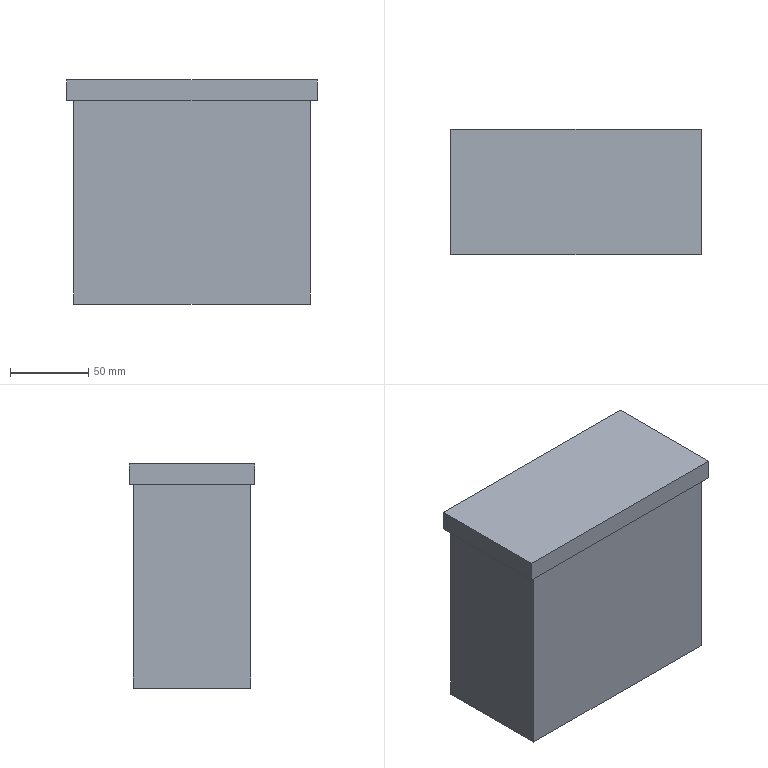Part | STEP file | NS-YB05C-A1 (five-digit digital display, with 232 interface) | 1 solid | 11 faces | box 160 x 80 x 143 mm | volume 1638650 mm3 | plane 11
STEP:
#1=CARTESIAN_POINT('',(0.,0.,0.));
#2=DIRECTION('',(0.,0.,1.));
#3=DIRECTION('',(1.,0.,0.));
#4=AXIS2_PLACEMENT_3D('',#1,#2,#3);
#5=CARTESIAN_POINT('',(-80.,40.,0.));
#6=VERTEX_POINT('',#5);
#7=CARTESIAN_POINT('',(-80.,-40.,0.));
#8=VERTEX_POINT('',#7);
#9=CARTESIAN_POINT('',(-80.,-40.,0.));
#10=DIRECTION('',(0.,-1.,0.));
#11=VECTOR('',#10,1.);
#12=LINE('',#9,#11);
#13=CARTESIAN_POINT('',(0.,0.,0.));
#14=DIRECTION('',(0.,0.,1.));
#15=DIRECTION('',(1.,0.,0.));
#16=AXIS2_PLACEMENT_3D('',#13,#14,#15);
#17=PLANE('',#16);
#18=CARTESIAN_POINT('',(-80.,-40.));
#19=DIRECTION('',(0.,-1.));
#20=VECTOR('',#19,1.);
#21=LINE('',#18,#20);
#22=(GEOMETRIC_REPRESENTATION_CONTEXT(2)PARAMETRIC_REPRESENTATION_CONTEXT()REPRESENTATION_CONTEXT('',''));
#23=DEFINITIONAL_REPRESENTATION('',(#21),#22);
#24=PCURVE('',#17,#23);
#25=CARTESIAN_POINT('',(-80.,-40.,13.));
#26=DIRECTION('',(1.,0.,0.));
#27=DIRECTION('',(0.,0.,-1.));
#28=AXIS2_PLACEMENT_3D('',#25,#26,#27);
#29=PLANE('',#28);
#30=CARTESIAN_POINT('',(13.,0.));
#31=DIRECTION('',(0.,-1.));
#32=VECTOR('',#31,1.);
#33=LINE('',#30,#32);
#34=(GEOMETRIC_REPRESENTATION_CONTEXT(2)PARAMETRIC_REPRESENTATION_CONTEXT()REPRESENTATION_CONTEXT('',''));
#35=DEFINITIONAL_REPRESENTATION('',(#33),#34);
#36=PCURVE('',#29,#35);
#37=SURFACE_CURVE('',#12,(#24,#36),.PCURVE_S1.);
#38=EDGE_CURVE('',#6,#8,#37,.T.);
#39=ORIENTED_EDGE('',*,*,#38,.F.);
#40=CARTESIAN_POINT('',(80.,40.,0.));
#41=VERTEX_POINT('',#40);
#42=CARTESIAN_POINT('',(80.,40.,0.));
#43=DIRECTION('',(-1.,0.,0.));
#44=VECTOR('',#43,1.);
#45=LINE('',#42,#44);
#46=CARTESIAN_POINT('',(80.,40.));
#47=DIRECTION('',(-1.,0.));
#48=VECTOR('',#47,1.);
#49=LINE('',#46,#48);
#50=(GEOMETRIC_REPRESENTATION_CONTEXT(2)PARAMETRIC_REPRESENTATION_CONTEXT()REPRESENTATION_CONTEXT('',''));
#51=DEFINITIONAL_REPRESENTATION('',(#49),#50);
#52=PCURVE('',#17,#51);
#53=CARTESIAN_POINT('',(80.,40.,13.));
#54=DIRECTION('',(0.,-1.,0.));
#55=DIRECTION('',(1.,0.,0.));
#56=AXIS2_PLACEMENT_3D('',#53,#54,#55);
#57=PLANE('',#56);
#58=CARTESIAN_POINT('',(0.,-13.));
#59=DIRECTION('',(-1.,0.));
#60=VECTOR('',#59,1.);
#61=LINE('',#58,#60);
#62=(GEOMETRIC_REPRESENTATION_CONTEXT(2)PARAMETRIC_REPRESENTATION_CONTEXT()REPRESENTATION_CONTEXT('',''));
#63=DEFINITIONAL_REPRESENTATION('',(#61),#62);
#64=PCURVE('',#57,#63);
#65=SURFACE_CURVE('',#45,(#52,#64),.PCURVE_S1.);
#66=EDGE_CURVE('',#41,#6,#65,.T.);
#67=ORIENTED_EDGE('',*,*,#66,.F.);
#68=CARTESIAN_POINT('',(80.,-40.,0.));
#69=VERTEX_POINT('',#68);
#70=CARTESIAN_POINT('',(80.,-40.,0.));
#71=DIRECTION('',(0.,1.,0.));
#72=VECTOR('',#71,1.);
#73=LINE('',#70,#72);
#74=CARTESIAN_POINT('',(80.,-40.));
#75=DIRECTION('',(0.,1.));
#76=VECTOR('',#75,1.);
#77=LINE('',#74,#76);
#78=(GEOMETRIC_REPRESENTATION_CONTEXT(2)PARAMETRIC_REPRESENTATION_CONTEXT()REPRESENTATION_CONTEXT('',''));
#79=DEFINITIONAL_REPRESENTATION('',(#77),#78);
#80=PCURVE('',#17,#79);
#81=CARTESIAN_POINT('',(80.,-40.,13.));
#82=DIRECTION('',(-1.,0.,0.));
#83=DIRECTION('',(0.,0.,1.));
#84=AXIS2_PLACEMENT_3D('',#81,#82,#83);
#85=PLANE('',#84);
#86=CARTESIAN_POINT('',(-13.,0.));
#87=DIRECTION('',(0.,1.));
#88=VECTOR('',#87,1.);
#89=LINE('',#86,#88);
#90=(GEOMETRIC_REPRESENTATION_CONTEXT(2)PARAMETRIC_REPRESENTATION_CONTEXT()REPRESENTATION_CONTEXT('',''));
#91=DEFINITIONAL_REPRESENTATION('',(#89),#90);
#92=PCURVE('',#85,#91);
#93=SURFACE_CURVE('',#73,(#80,#92),.PCURVE_S1.);
#94=EDGE_CURVE('',#69,#41,#93,.T.);
#95=ORIENTED_EDGE('',*,*,#94,.F.);
#96=CARTESIAN_POINT('',(80.,-40.,0.));
#97=DIRECTION('',(1.,0.,0.));
#98=VECTOR('',#97,1.);
#99=LINE('',#96,#98);
#100=CARTESIAN_POINT('',(80.,-40.));
#101=DIRECTION('',(1.,0.));
#102=VECTOR('',#101,1.);
#103=LINE('',#100,#102);
#104=(GEOMETRIC_REPRESENTATION_CONTEXT(2)PARAMETRIC_REPRESENTATION_CONTEXT()REPRESENTATION_CONTEXT('',''));
#105=DEFINITIONAL_REPRESENTATION('',(#103),#104);
#106=PCURVE('',#17,#105);
#107=CARTESIAN_POINT('',(80.,-40.,13.));
#108=DIRECTION('',(0.,1.,0.));
#109=DIRECTION('',(-1.,0.,0.));
#110=AXIS2_PLACEMENT_3D('',#107,#108,#109);
#111=PLANE('',#110);
#112=CARTESIAN_POINT('',(0.,-13.));
#113=DIRECTION('',(-1.,0.));
#114=VECTOR('',#113,1.);
#115=LINE('',#112,#114);
#116=(GEOMETRIC_REPRESENTATION_CONTEXT(2)PARAMETRIC_REPRESENTATION_CONTEXT()REPRESENTATION_CONTEXT('',''));
#117=DEFINITIONAL_REPRESENTATION('',(#115),#116);
#118=PCURVE('',#111,#117);
#119=SURFACE_CURVE('',#99,(#106,#118),.PCURVE_S1.);
#120=EDGE_CURVE('',#8,#69,#119,.T.);
#121=ORIENTED_EDGE('',*,*,#120,.F.);
#122=EDGE_LOOP('',(#39,#67,#95,#121));
#123=FACE_BOUND('',#122,.T.);
#124=CARTESIAN_POINT('',(75.5,37.5,0.));
#125=VERTEX_POINT('',#124);
#126=CARTESIAN_POINT('',(75.5,-37.5,0.));
#127=VERTEX_POINT('',#126);
#128=CARTESIAN_POINT('',(75.5,-37.5,0.));
#129=DIRECTION('',(0.,-1.,0.));
#130=VECTOR('',#129,1.);
#131=LINE('',#128,#130);
#132=CARTESIAN_POINT('',(75.5,-37.5));
#133=DIRECTION('',(0.,-1.));
#134=VECTOR('',#133,1.);
#135=LINE('',#132,#134);
#136=(GEOMETRIC_REPRESENTATION_CONTEXT(2)PARAMETRIC_REPRESENTATION_CONTEXT()REPRESENTATION_CONTEXT('',''));
#137=DEFINITIONAL_REPRESENTATION('',(#135),#136);
#138=PCURVE('',#17,#137);
#139=CARTESIAN_POINT('',(75.5,-37.5,-130.));
#140=DIRECTION('',(-1.,0.,0.));
#141=DIRECTION('',(0.,0.,1.));
#142=AXIS2_PLACEMENT_3D('',#139,#140,#141);
#143=PLANE('',#142);
#144=CARTESIAN_POINT('',(130.,0.));
#145=DIRECTION('',(0.,-1.));
#146=VECTOR('',#145,1.);
#147=LINE('',#144,#146);
#148=(GEOMETRIC_REPRESENTATION_CONTEXT(2)PARAMETRIC_REPRESENTATION_CONTEXT()REPRESENTATION_CONTEXT('',''));
#149=DEFINITIONAL_REPRESENTATION('',(#147),#148);
#150=PCURVE('',#143,#149);
#151=SURFACE_CURVE('',#131,(#138,#150),.PCURVE_S1.);
#152=EDGE_CURVE('',#125,#127,#151,.T.);
#153=ORIENTED_EDGE('',*,*,#152,.F.);
#154=CARTESIAN_POINT('',(-75.5,37.5,0.));
#155=VERTEX_POINT('',#154);
#156=CARTESIAN_POINT('',(-75.5,37.5,0.));
#157=DIRECTION('',(1.,0.,0.));
#158=VECTOR('',#157,1.);
#159=LINE('',#156,#158);
#160=CARTESIAN_POINT('',(-75.5,37.5));
#161=DIRECTION('',(1.,0.));
#162=VECTOR('',#161,1.);
#163=LINE('',#160,#162);
#164=(GEOMETRIC_REPRESENTATION_CONTEXT(2)PARAMETRIC_REPRESENTATION_CONTEXT()REPRESENTATION_CONTEXT('',''));
#165=DEFINITIONAL_REPRESENTATION('',(#163),#164);
#166=PCURVE('',#17,#165);
#167=CARTESIAN_POINT('',(-75.5,37.5,-130.));
#168=DIRECTION('',(0.,-1.,0.));
#169=DIRECTION('',(1.,0.,0.));
#170=AXIS2_PLACEMENT_3D('',#167,#168,#169);
#171=PLANE('',#170);
#172=CARTESIAN_POINT('',(0.,130.));
#173=DIRECTION('',(1.,0.));
#174=VECTOR('',#173,1.);
#175=LINE('',#172,#174);
#176=(GEOMETRIC_REPRESENTATION_CONTEXT(2)PARAMETRIC_REPRESENTATION_CONTEXT()REPRESENTATION_CONTEXT('',''));
#177=DEFINITIONAL_REPRESENTATION('',(#175),#176);
#178=PCURVE('',#171,#177);
#179=SURFACE_CURVE('',#159,(#166,#178),.PCURVE_S1.);
#180=EDGE_CURVE('',#155,#125,#179,.T.);
#181=ORIENTED_EDGE('',*,*,#180,.F.);
#182=CARTESIAN_POINT('',(-75.5,-37.5,0.));
#183=VERTEX_POINT('',#182);
#184=CARTESIAN_POINT('',(-75.5,-37.5,0.));
#185=DIRECTION('',(0.,1.,0.));
#186=VECTOR('',#185,1.);
#187=LINE('',#184,#186);
#188=CARTESIAN_POINT('',(-75.5,-37.5));
#189=DIRECTION('',(0.,1.));
#190=VECTOR('',#189,1.);
#191=LINE('',#188,#190);
#192=(GEOMETRIC_REPRESENTATION_CONTEXT(2)PARAMETRIC_REPRESENTATION_CONTEXT()REPRESENTATION_CONTEXT('',''));
#193=DEFINITIONAL_REPRESENTATION('',(#191),#192);
#194=PCURVE('',#17,#193);
#195=CARTESIAN_POINT('',(-75.5,-37.5,-130.));
#196=DIRECTION('',(1.,0.,0.));
#197=DIRECTION('',(0.,0.,-1.));
#198=AXIS2_PLACEMENT_3D('',#195,#196,#197);
#199=PLANE('',#198);
#200=CARTESIAN_POINT('',(-130.,0.));
#201=DIRECTION('',(0.,1.));
#202=VECTOR('',#201,1.);
#203=LINE('',#200,#202);
#204=(GEOMETRIC_REPRESENTATION_CONTEXT(2)PARAMETRIC_REPRESENTATION_CONTEXT()REPRESENTATION_CONTEXT('',''));
#205=DEFINITIONAL_REPRESENTATION('',(#203),#204);
#206=PCURVE('',#199,#205);
#207=SURFACE_CURVE('',#187,(#194,#206),.PCURVE_S1.);
#208=EDGE_CURVE('',#183,#155,#207,.T.);
#209=ORIENTED_EDGE('',*,*,#208,.F.);
#210=CARTESIAN_POINT('',(-75.5,-37.5,0.));
#211=DIRECTION('',(-1.,0.,0.));
#212=VECTOR('',#211,1.);
#213=LINE('',#210,#212);
#214=CARTESIAN_POINT('',(-75.5,-37.5));
#215=DIRECTION('',(-1.,0.));
#216=VECTOR('',#215,1.);
#217=LINE('',#214,#216);
#218=(GEOMETRIC_REPRESENTATION_CONTEXT(2)PARAMETRIC_REPRESENTATION_CONTEXT()REPRESENTATION_CONTEXT('',''));
#219=DEFINITIONAL_REPRESENTATION('',(#217),#218);
#220=PCURVE('',#17,#219);
#221=CARTESIAN_POINT('',(-75.5,-37.5,-130.));
#222=DIRECTION('',(0.,1.,0.));
#223=DIRECTION('',(-1.,0.,0.));
#224=AXIS2_PLACEMENT_3D('',#221,#222,#223);
#225=PLANE('',#224);
#226=CARTESIAN_POINT('',(0.,130.));
#227=DIRECTION('',(1.,0.));
#228=VECTOR('',#227,1.);
#229=LINE('',#226,#228);
#230=(GEOMETRIC_REPRESENTATION_CONTEXT(2)PARAMETRIC_REPRESENTATION_CONTEXT()REPRESENTATION_CONTEXT('',''));
#231=DEFINITIONAL_REPRESENTATION('',(#229),#230);
#232=PCURVE('',#225,#231);
#233=SURFACE_CURVE('',#213,(#220,#232),.PCURVE_S1.);
#234=EDGE_CURVE('',#127,#183,#233,.T.);
#235=ORIENTED_EDGE('',*,*,#234,.F.);
#236=EDGE_LOOP('',(#153,#181,#209,#235));
#237=FACE_BOUND('',#236,.T.);
#238=ADVANCED_FACE('',(#123,#237),#17,.F.);
#239=ORIENTED_EDGE('',*,*,#38,.T.);
#240=CARTESIAN_POINT('',(-80.,-40.,13.));
#241=VERTEX_POINT('',#240);
#242=CARTESIAN_POINT('',(-80.,-40.,13.));
#243=DIRECTION('',(0.,0.,-1.));
#244=VECTOR('',#243,1.);
#245=LINE('',#242,#244);
#246=CARTESIAN_POINT('',(0.,0.));
#247=DIRECTION('',(1.,0.));
#248=VECTOR('',#247,1.);
#249=LINE('',#246,#248);
#250=(GEOMETRIC_REPRESENTATION_CONTEXT(2)PARAMETRIC_REPRESENTATION_CONTEXT()REPRESENTATION_CONTEXT('',''));
#251=DEFINITIONAL_REPRESENTATION('',(#249),#250);
#252=PCURVE('',#29,#251);
#253=CARTESIAN_POINT('',(160.,0.));
#254=DIRECTION('',(0.,-1.));
#255=VECTOR('',#254,1.);
#256=LINE('',#253,#255);
#257=(GEOMETRIC_REPRESENTATION_CONTEXT(2)PARAMETRIC_REPRESENTATION_CONTEXT()REPRESENTATION_CONTEXT('',''));
#258=DEFINITIONAL_REPRESENTATION('',(#256),#257);
#259=PCURVE('',#111,#258);
#260=SURFACE_CURVE('',#245,(#252,#259),.PCURVE_S1.);
#261=EDGE_CURVE('',#241,#8,#260,.T.);
#262=ORIENTED_EDGE('',*,*,#261,.F.);
#263=CARTESIAN_POINT('',(-80.,40.,13.));
#264=VERTEX_POINT('',#263);
#265=CARTESIAN_POINT('',(-80.,-40.,13.));
#266=DIRECTION('',(0.,-1.,0.));
#267=VECTOR('',#266,1.);
#268=LINE('',#265,#267);
#269=CARTESIAN_POINT('',(0.,0.));
#270=DIRECTION('',(0.,-1.));
#271=VECTOR('',#270,1.);
#272=LINE('',#269,#271);
#273=(GEOMETRIC_REPRESENTATION_CONTEXT(2)PARAMETRIC_REPRESENTATION_CONTEXT()REPRESENTATION_CONTEXT('',''));
#274=DEFINITIONAL_REPRESENTATION('',(#272),#273);
#275=PCURVE('',#29,#274);
#276=CARTESIAN_POINT('',(0.,0.,13.));
#277=DIRECTION('',(0.,0.,1.));
#278=DIRECTION('',(1.,0.,0.));
#279=AXIS2_PLACEMENT_3D('',#276,#277,#278);
#280=PLANE('',#279);
#281=CARTESIAN_POINT('',(-80.,-40.));
#282=DIRECTION('',(0.,-1.));
#283=VECTOR('',#282,1.);
#284=LINE('',#281,#283);
#285=(GEOMETRIC_REPRESENTATION_CONTEXT(2)PARAMETRIC_REPRESENTATION_CONTEXT()REPRESENTATION_CONTEXT('',''));
#286=DEFINITIONAL_REPRESENTATION('',(#284),#285);
#287=PCURVE('',#280,#286);
#288=SURFACE_CURVE('',#268,(#275,#287),.PCURVE_S1.);
#289=EDGE_CURVE('',#264,#241,#288,.T.);
#290=ORIENTED_EDGE('',*,*,#289,.F.);
#291=CARTESIAN_POINT('',(-80.,40.,13.));
#292=DIRECTION('',(0.,0.,-1.));
#293=VECTOR('',#292,1.);
#294=LINE('',#291,#293);
#295=CARTESIAN_POINT('',(0.,80.));
#296=DIRECTION('',(1.,0.));
#297=VECTOR('',#296,1.);
#298=LINE('',#295,#297);
#299=(GEOMETRIC_REPRESENTATION_CONTEXT(2)PARAMETRIC_REPRESENTATION_CONTEXT()REPRESENTATION_CONTEXT('',''));
#300=DEFINITIONAL_REPRESENTATION('',(#298),#299);
#301=PCURVE('',#29,#300);
#302=CARTESIAN_POINT('',(-160.,0.));
#303=DIRECTION('',(0.,-1.));
#304=VECTOR('',#303,1.);
#305=LINE('',#302,#304);
#306=(GEOMETRIC_REPRESENTATION_CONTEXT(2)PARAMETRIC_REPRESENTATION_CONTEXT()REPRESENTATION_CONTEXT('',''));
#307=DEFINITIONAL_REPRESENTATION('',(#305),#306);
#308=PCURVE('',#57,#307);
#309=SURFACE_CURVE('',#294,(#301,#308),.PCURVE_S1.);
#310=EDGE_CURVE('',#264,#6,#309,.T.);
#311=ORIENTED_EDGE('',*,*,#310,.T.);
#312=EDGE_LOOP('',(#239,#262,#290,#311));
#313=FACE_BOUND('',#312,.T.);
#314=ADVANCED_FACE('',(#313),#29,.F.);
#315=ORIENTED_EDGE('',*,*,#120,.T.);
#316=CARTESIAN_POINT('',(80.,-40.,13.));
#317=VERTEX_POINT('',#316);
#318=CARTESIAN_POINT('',(80.,-40.,13.));
#319=DIRECTION('',(0.,0.,-1.));
#320=VECTOR('',#319,1.);
#321=LINE('',#318,#320);
#322=CARTESIAN_POINT('',(0.,0.));
#323=DIRECTION('',(0.,-1.));
#324=VECTOR('',#323,1.);
#325=LINE('',#322,#324);
#326=(GEOMETRIC_REPRESENTATION_CONTEXT(2)PARAMETRIC_REPRESENTATION_CONTEXT()REPRESENTATION_CONTEXT('',''));
#327=DEFINITIONAL_REPRESENTATION('',(#325),#326);
#328=PCURVE('',#111,#327);
#329=CARTESIAN_POINT('',(0.,0.));
#330=DIRECTION('',(-1.,0.));
#331=VECTOR('',#330,1.);
#332=LINE('',#329,#331);
#333=(GEOMETRIC_REPRESENTATION_CONTEXT(2)PARAMETRIC_REPRESENTATION_CONTEXT()REPRESENTATION_CONTEXT('',''));
#334=DEFINITIONAL_REPRESENTATION('',(#332),#333);
#335=PCURVE('',#85,#334);
#336=SURFACE_CURVE('',#321,(#328,#335),.PCURVE_S1.);
#337=EDGE_CURVE('',#317,#69,#336,.T.);
#338=ORIENTED_EDGE('',*,*,#337,.F.);
#339=CARTESIAN_POINT('',(80.,-40.,13.));
#340=DIRECTION('',(1.,0.,0.));
#341=VECTOR('',#340,1.);
#342=LINE('',#339,#341);
#343=CARTESIAN_POINT('',(0.,0.));
#344=DIRECTION('',(-1.,0.));
#345=VECTOR('',#344,1.);
#346=LINE('',#343,#345);
#347=(GEOMETRIC_REPRESENTATION_CONTEXT(2)PARAMETRIC_REPRESENTATION_CONTEXT()REPRESENTATION_CONTEXT('',''));
#348=DEFINITIONAL_REPRESENTATION('',(#346),#347);
#349=PCURVE('',#111,#348);
#350=CARTESIAN_POINT('',(80.,-40.));
#351=DIRECTION('',(1.,0.));
#352=VECTOR('',#351,1.);
#353=LINE('',#350,#352);
#354=(GEOMETRIC_REPRESENTATION_CONTEXT(2)PARAMETRIC_REPRESENTATION_CONTEXT()REPRESENTATION_CONTEXT('',''));
#355=DEFINITIONAL_REPRESENTATION('',(#353),#354);
#356=PCURVE('',#280,#355);
#357=SURFACE_CURVE('',#342,(#349,#356),.PCURVE_S1.);
#358=EDGE_CURVE('',#241,#317,#357,.T.);
#359=ORIENTED_EDGE('',*,*,#358,.F.);
#360=ORIENTED_EDGE('',*,*,#261,.T.);
#361=EDGE_LOOP('',(#315,#338,#359,#360));
#362=FACE_BOUND('',#361,.T.);
#363=ADVANCED_FACE('',(#362),#111,.F.);
#364=ORIENTED_EDGE('',*,*,#94,.T.);
#365=CARTESIAN_POINT('',(80.,40.,13.));
#366=VERTEX_POINT('',#365);
#367=CARTESIAN_POINT('',(80.,40.,13.));
#368=DIRECTION('',(0.,0.,-1.));
#369=VECTOR('',#368,1.);
#370=LINE('',#367,#369);
#371=CARTESIAN_POINT('',(0.,80.));
#372=DIRECTION('',(-1.,0.));
#373=VECTOR('',#372,1.);
#374=LINE('',#371,#373);
#375=(GEOMETRIC_REPRESENTATION_CONTEXT(2)PARAMETRIC_REPRESENTATION_CONTEXT()REPRESENTATION_CONTEXT('',''));
#376=DEFINITIONAL_REPRESENTATION('',(#374),#375);
#377=PCURVE('',#85,#376);
#378=CARTESIAN_POINT('',(0.,0.));
#379=DIRECTION('',(0.,-1.));
#380=VECTOR('',#379,1.);
#381=LINE('',#378,#380);
#382=(GEOMETRIC_REPRESENTATION_CONTEXT(2)PARAMETRIC_REPRESENTATION_CONTEXT()REPRESENTATION_CONTEXT('',''));
#383=DEFINITIONAL_REPRESENTATION('',(#381),#382);
#384=PCURVE('',#57,#383);
#385=SURFACE_CURVE('',#370,(#377,#384),.PCURVE_S1.);
#386=EDGE_CURVE('',#366,#41,#385,.T.);
#387=ORIENTED_EDGE('',*,*,#386,.F.);
#388=CARTESIAN_POINT('',(80.,-40.,13.));
#389=DIRECTION('',(0.,1.,0.));
#390=VECTOR('',#389,1.);
#391=LINE('',#388,#390);
#392=CARTESIAN_POINT('',(0.,0.));
#393=DIRECTION('',(0.,1.));
#394=VECTOR('',#393,1.);
#395=LINE('',#392,#394);
#396=(GEOMETRIC_REPRESENTATION_CONTEXT(2)PARAMETRIC_REPRESENTATION_CONTEXT()REPRESENTATION_CONTEXT('',''));
#397=DEFINITIONAL_REPRESENTATION('',(#395),#396);
#398=PCURVE('',#85,#397);
#399=CARTESIAN_POINT('',(80.,-40.));
#400=DIRECTION('',(0.,1.));
#401=VECTOR('',#400,1.);
#402=LINE('',#399,#401);
#403=(GEOMETRIC_REPRESENTATION_CONTEXT(2)PARAMETRIC_REPRESENTATION_CONTEXT()REPRESENTATION_CONTEXT('',''));
#404=DEFINITIONAL_REPRESENTATION('',(#402),#403);
#405=PCURVE('',#280,#404);
#406=SURFACE_CURVE('',#391,(#398,#405),.PCURVE_S1.);
#407=EDGE_CURVE('',#317,#366,#406,.T.);
#408=ORIENTED_EDGE('',*,*,#407,.F.);
#409=ORIENTED_EDGE('',*,*,#337,.T.);
#410=EDGE_LOOP('',(#364,#387,#408,#409));
#411=FACE_BOUND('',#410,.T.);
#412=ADVANCED_FACE('',(#411),#85,.F.);
#413=ORIENTED_EDGE('',*,*,#66,.T.);
#414=ORIENTED_EDGE('',*,*,#310,.F.);
#415=CARTESIAN_POINT('',(80.,40.,13.));
#416=DIRECTION('',(-1.,0.,0.));
#417=VECTOR('',#416,1.);
#418=LINE('',#415,#417);
#419=CARTESIAN_POINT('',(0.,0.));
#420=DIRECTION('',(-1.,0.));
#421=VECTOR('',#420,1.);
#422=LINE('',#419,#421);
#423=(GEOMETRIC_REPRESENTATION_CONTEXT(2)PARAMETRIC_REPRESENTATION_CONTEXT()REPRESENTATION_CONTEXT('',''));
#424=DEFINITIONAL_REPRESENTATION('',(#422),#423);
#425=PCURVE('',#57,#424);
#426=CARTESIAN_POINT('',(80.,40.));
#427=DIRECTION('',(-1.,0.));
#428=VECTOR('',#427,1.);
#429=LINE('',#426,#428);
#430=(GEOMETRIC_REPRESENTATION_CONTEXT(2)PARAMETRIC_REPRESENTATION_CONTEXT()REPRESENTATION_CONTEXT('',''));
#431=DEFINITIONAL_REPRESENTATION('',(#429),#430);
#432=PCURVE('',#280,#431);
#433=SURFACE_CURVE('',#418,(#425,#432),.PCURVE_S1.);
#434=EDGE_CURVE('',#366,#264,#433,.T.);
#435=ORIENTED_EDGE('',*,*,#434,.F.);
#436=ORIENTED_EDGE('',*,*,#386,.T.);
#437=EDGE_LOOP('',(#413,#414,#435,#436));
#438=FACE_BOUND('',#437,.T.);
#439=ADVANCED_FACE('',(#438),#57,.F.);
#440=ORIENTED_EDGE('',*,*,#289,.T.);
#441=ORIENTED_EDGE('',*,*,#358,.T.);
#442=ORIENTED_EDGE('',*,*,#407,.T.);
#443=ORIENTED_EDGE('',*,*,#434,.T.);
#444=EDGE_LOOP('',(#440,#441,#442,#443));
#445=FACE_BOUND('',#444,.T.);
#446=ADVANCED_FACE('',(#445),#280,.T.);
#447=ORIENTED_EDGE('',*,*,#152,.T.);
#448=CARTESIAN_POINT('',(75.5,-37.5,-130.));
#449=VERTEX_POINT('',#448);
#450=CARTESIAN_POINT('',(75.5,-37.5,-130.));
#451=DIRECTION('',(0.,0.,1.));
#452=VECTOR('',#451,1.);
#453=LINE('',#450,#452);
#454=CARTESIAN_POINT('',(0.,0.));
#455=DIRECTION('',(1.,0.));
#456=VECTOR('',#455,1.);
#457=LINE('',#454,#456);
#458=(GEOMETRIC_REPRESENTATION_CONTEXT(2)PARAMETRIC_REPRESENTATION_CONTEXT()REPRESENTATION_CONTEXT('',''));
#459=DEFINITIONAL_REPRESENTATION('',(#457),#458);
#460=PCURVE('',#143,#459);
#461=CARTESIAN_POINT('',(-151.,0.));
#462=DIRECTION('',(0.,1.));
#463=VECTOR('',#462,1.);
#464=LINE('',#461,#463);
#465=(GEOMETRIC_REPRESENTATION_CONTEXT(2)PARAMETRIC_REPRESENTATION_CONTEXT()REPRESENTATION_CONTEXT('',''));
#466=DEFINITIONAL_REPRESENTATION('',(#464),#465);
#467=PCURVE('',#225,#466);
#468=SURFACE_CURVE('',#453,(#460,#467),.PCURVE_S1.);
#469=EDGE_CURVE('',#449,#127,#468,.T.);
#470=ORIENTED_EDGE('',*,*,#469,.F.);
#471=CARTESIAN_POINT('',(75.5,37.5,-130.));
#472=VERTEX_POINT('',#471);
#473=CARTESIAN_POINT('',(75.5,-37.5,-130.));
#474=DIRECTION('',(0.,-1.,0.));
#475=VECTOR('',#474,1.);
#476=LINE('',#473,#475);
#477=CARTESIAN_POINT('',(0.,0.));
#478=DIRECTION('',(0.,-1.));
#479=VECTOR('',#478,1.);
#480=LINE('',#477,#479);
#481=(GEOMETRIC_REPRESENTATION_CONTEXT(2)PARAMETRIC_REPRESENTATION_CONTEXT()REPRESENTATION_CONTEXT('',''));
#482=DEFINITIONAL_REPRESENTATION('',(#480),#481);
#483=PCURVE('',#143,#482);
#484=CARTESIAN_POINT('',(0.,0.,-130.));
#485=DIRECTION('',(0.,0.,-1.));
#486=DIRECTION('',(-1.,0.,0.));
#487=AXIS2_PLACEMENT_3D('',#484,#485,#486);
#488=PLANE('',#487);
#489=CARTESIAN_POINT('',(-75.5,-37.5));
#490=DIRECTION('',(0.,-1.));
#491=VECTOR('',#490,1.);
#492=LINE('',#489,#491);
#493=(GEOMETRIC_REPRESENTATION_CONTEXT(2)PARAMETRIC_REPRESENTATION_CONTEXT()REPRESENTATION_CONTEXT('',''));
#494=DEFINITIONAL_REPRESENTATION('',(#492),#493);
#495=PCURVE('',#488,#494);
#496=SURFACE_CURVE('',#476,(#483,#495),.PCURVE_S1.);
#497=EDGE_CURVE('',#472,#449,#496,.T.);
#498=ORIENTED_EDGE('',*,*,#497,.F.);
#499=CARTESIAN_POINT('',(75.5,37.5,-130.));
#500=DIRECTION('',(0.,0.,1.));
#501=VECTOR('',#500,1.);
#502=LINE('',#499,#501);
#503=CARTESIAN_POINT('',(0.,75.));
#504=DIRECTION('',(1.,0.));
#505=VECTOR('',#504,1.);
#506=LINE('',#503,#505);
#507=(GEOMETRIC_REPRESENTATION_CONTEXT(2)PARAMETRIC_REPRESENTATION_CONTEXT()REPRESENTATION_CONTEXT('',''));
#508=DEFINITIONAL_REPRESENTATION('',(#506),#507);
#509=PCURVE('',#143,#508);
#510=CARTESIAN_POINT('',(151.,0.));
#511=DIRECTION('',(0.,1.));
#512=VECTOR('',#511,1.);
#513=LINE('',#510,#512);
#514=(GEOMETRIC_REPRESENTATION_CONTEXT(2)PARAMETRIC_REPRESENTATION_CONTEXT()REPRESENTATION_CONTEXT('',''));
#515=DEFINITIONAL_REPRESENTATION('',(#513),#514);
#516=PCURVE('',#171,#515);
#517=SURFACE_CURVE('',#502,(#509,#516),.PCURVE_S1.);
#518=EDGE_CURVE('',#472,#125,#517,.T.);
#519=ORIENTED_EDGE('',*,*,#518,.T.);
#520=EDGE_LOOP('',(#447,#470,#498,#519));
#521=FACE_BOUND('',#520,.T.);
#522=ADVANCED_FACE('',(#521),#143,.F.);
#523=ORIENTED_EDGE('',*,*,#234,.T.);
#524=CARTESIAN_POINT('',(-75.5,-37.5,-130.));
#525=VERTEX_POINT('',#524);
#526=CARTESIAN_POINT('',(-75.5,-37.5,-130.));
#527=DIRECTION('',(0.,0.,1.));
#528=VECTOR('',#527,1.);
#529=LINE('',#526,#528);
#530=CARTESIAN_POINT('',(0.,0.));
#531=DIRECTION('',(0.,1.));
#532=VECTOR('',#531,1.);
#533=LINE('',#530,#532);
#534=(GEOMETRIC_REPRESENTATION_CONTEXT(2)PARAMETRIC_REPRESENTATION_CONTEXT()REPRESENTATION_CONTEXT('',''));
#535=DEFINITIONAL_REPRESENTATION('',(#533),#534);
#536=PCURVE('',#225,#535);
#537=CARTESIAN_POINT('',(0.,0.));
#538=DIRECTION('',(-1.,0.));
#539=VECTOR('',#538,1.);
#540=LINE('',#537,#539);
#541=(GEOMETRIC_REPRESENTATION_CONTEXT(2)PARAMETRIC_REPRESENTATION_CONTEXT()REPRESENTATION_CONTEXT('',''));
#542=DEFINITIONAL_REPRESENTATION('',(#540),#541);
#543=PCURVE('',#199,#542);
#544=SURFACE_CURVE('',#529,(#536,#543),.PCURVE_S1.);
#545=EDGE_CURVE('',#525,#183,#544,.T.);
#546=ORIENTED_EDGE('',*,*,#545,.F.);
#547=CARTESIAN_POINT('',(-75.5,-37.5,-130.));
#548=DIRECTION('',(-1.,0.,0.));
#549=VECTOR('',#548,1.);
#550=LINE('',#547,#549);
#551=CARTESIAN_POINT('',(0.,0.));
#552=DIRECTION('',(1.,0.));
#553=VECTOR('',#552,1.);
#554=LINE('',#551,#553);
#555=(GEOMETRIC_REPRESENTATION_CONTEXT(2)PARAMETRIC_REPRESENTATION_CONTEXT()REPRESENTATION_CONTEXT('',''));
#556=DEFINITIONAL_REPRESENTATION('',(#554),#555);
#557=PCURVE('',#225,#556);
#558=CARTESIAN_POINT('',(75.5,-37.5));
#559=DIRECTION('',(1.,0.));
#560=VECTOR('',#559,1.);
#561=LINE('',#558,#560);
#562=(GEOMETRIC_REPRESENTATION_CONTEXT(2)PARAMETRIC_REPRESENTATION_CONTEXT()REPRESENTATION_CONTEXT('',''));
#563=DEFINITIONAL_REPRESENTATION('',(#561),#562);
#564=PCURVE('',#488,#563);
#565=SURFACE_CURVE('',#550,(#557,#564),.PCURVE_S1.);
#566=EDGE_CURVE('',#449,#525,#565,.T.);
#567=ORIENTED_EDGE('',*,*,#566,.F.);
#568=ORIENTED_EDGE('',*,*,#469,.T.);
#569=EDGE_LOOP('',(#523,#546,#567,#568));
#570=FACE_BOUND('',#569,.T.);
#571=ADVANCED_FACE('',(#570),#225,.F.);
#572=ORIENTED_EDGE('',*,*,#208,.T.);
#573=CARTESIAN_POINT('',(-75.5,37.5,-130.));
#574=VERTEX_POINT('',#573);
#575=CARTESIAN_POINT('',(-75.5,37.5,-130.));
#576=DIRECTION('',(0.,0.,1.));
#577=VECTOR('',#576,1.);
#578=LINE('',#575,#577);
#579=CARTESIAN_POINT('',(0.,75.));
#580=DIRECTION('',(-1.,0.));
#581=VECTOR('',#580,1.);
#582=LINE('',#579,#581);
#583=(GEOMETRIC_REPRESENTATION_CONTEXT(2)PARAMETRIC_REPRESENTATION_CONTEXT()REPRESENTATION_CONTEXT('',''));
#584=DEFINITIONAL_REPRESENTATION('',(#582),#583);
#585=PCURVE('',#199,#584);
#586=CARTESIAN_POINT('',(0.,0.));
#587=DIRECTION('',(0.,1.));
#588=VECTOR('',#587,1.);
#589=LINE('',#586,#588);
#590=(GEOMETRIC_REPRESENTATION_CONTEXT(2)PARAMETRIC_REPRESENTATION_CONTEXT()REPRESENTATION_CONTEXT('',''));
#591=DEFINITIONAL_REPRESENTATION('',(#589),#590);
#592=PCURVE('',#171,#591);
#593=SURFACE_CURVE('',#578,(#585,#592),.PCURVE_S1.);
#594=EDGE_CURVE('',#574,#155,#593,.T.);
#595=ORIENTED_EDGE('',*,*,#594,.F.);
#596=CARTESIAN_POINT('',(-75.5,-37.5,-130.));
#597=DIRECTION('',(0.,1.,0.));
#598=VECTOR('',#597,1.);
#599=LINE('',#596,#598);
#600=CARTESIAN_POINT('',(0.,0.));
#601=DIRECTION('',(0.,1.));
#602=VECTOR('',#601,1.);
#603=LINE('',#600,#602);
#604=(GEOMETRIC_REPRESENTATION_CONTEXT(2)PARAMETRIC_REPRESENTATION_CONTEXT()REPRESENTATION_CONTEXT('',''));
#605=DEFINITIONAL_REPRESENTATION('',(#603),#604);
#606=PCURVE('',#199,#605);
#607=CARTESIAN_POINT('',(75.5,-37.5));
#608=DIRECTION('',(0.,1.));
#609=VECTOR('',#608,1.);
#610=LINE('',#607,#609);
#611=(GEOMETRIC_REPRESENTATION_CONTEXT(2)PARAMETRIC_REPRESENTATION_CONTEXT()REPRESENTATION_CONTEXT('',''));
#612=DEFINITIONAL_REPRESENTATION('',(#610),#611);
#613=PCURVE('',#488,#612);
#614=SURFACE_CURVE('',#599,(#606,#613),.PCURVE_S1.);
#615=EDGE_CURVE('',#525,#574,#614,.T.);
#616=ORIENTED_EDGE('',*,*,#615,.F.);
#617=ORIENTED_EDGE('',*,*,#545,.T.);
#618=EDGE_LOOP('',(#572,#595,#616,#617));
#619=FACE_BOUND('',#618,.T.);
#620=ADVANCED_FACE('',(#619),#199,.F.);
#621=ORIENTED_EDGE('',*,*,#180,.T.);
#622=ORIENTED_EDGE('',*,*,#518,.F.);
#623=CARTESIAN_POINT('',(-75.5,37.5,-130.));
#624=DIRECTION('',(1.,0.,0.));
#625=VECTOR('',#624,1.);
#626=LINE('',#623,#625);
#627=CARTESIAN_POINT('',(0.,0.));
#628=DIRECTION('',(1.,0.));
#629=VECTOR('',#628,1.);
#630=LINE('',#627,#629);
#631=(GEOMETRIC_REPRESENTATION_CONTEXT(2)PARAMETRIC_REPRESENTATION_CONTEXT()REPRESENTATION_CONTEXT('',''));
#632=DEFINITIONAL_REPRESENTATION('',(#630),#631);
#633=PCURVE('',#171,#632);
#634=CARTESIAN_POINT('',(75.5,37.5));
#635=DIRECTION('',(-1.,0.));
#636=VECTOR('',#635,1.);
#637=LINE('',#634,#636);
#638=(GEOMETRIC_REPRESENTATION_CONTEXT(2)PARAMETRIC_REPRESENTATION_CONTEXT()REPRESENTATION_CONTEXT('',''));
#639=DEFINITIONAL_REPRESENTATION('',(#637),#638);
#640=PCURVE('',#488,#639);
#641=SURFACE_CURVE('',#626,(#633,#640),.PCURVE_S1.);
#642=EDGE_CURVE('',#574,#472,#641,.T.);
#643=ORIENTED_EDGE('',*,*,#642,.F.);
#644=ORIENTED_EDGE('',*,*,#594,.T.);
#645=EDGE_LOOP('',(#621,#622,#643,#644));
#646=FACE_BOUND('',#645,.T.);
#647=ADVANCED_FACE('',(#646),#171,.F.);
#648=ORIENTED_EDGE('',*,*,#497,.T.);
#649=ORIENTED_EDGE('',*,*,#566,.T.);
#650=ORIENTED_EDGE('',*,*,#615,.T.);
#651=ORIENTED_EDGE('',*,*,#642,.T.);
#652=EDGE_LOOP('',(#648,#649,#650,#651));
#653=FACE_BOUND('',#652,.T.);
#654=ADVANCED_FACE('',(#653),#488,.T.);
#655=CLOSED_SHELL('',(#238,#314,#363,#412,#439,#446,#522,#571,#620,#647,#654));
#656=MANIFOLD_SOLID_BREP('',#655);
#657=(LENGTH_UNIT()NAMED_UNIT(*)SI_UNIT(.MILLI.,.METRE.));
#658=UNCERTAINTY_MEASURE_WITH_UNIT(LENGTH_MEASURE(0.0000001),#657,'','');
#659=(NAMED_UNIT(*)PLANE_ANGLE_UNIT()SI_UNIT($,.RADIAN.));
#660=(NAMED_UNIT(*)SI_UNIT($,.STERADIAN.)SOLID_ANGLE_UNIT());
#661=(GEOMETRIC_REPRESENTATION_CONTEXT(3)GLOBAL_UNCERTAINTY_ASSIGNED_CONTEXT((#658))GLOBAL_UNIT_ASSIGNED_CONTEXT((#657,#659,#660))REPRESENTATION_CONTEXT('',''));
#662=ADVANCED_BREP_SHAPE_REPRESENTATION('',(#4,#656),#661);